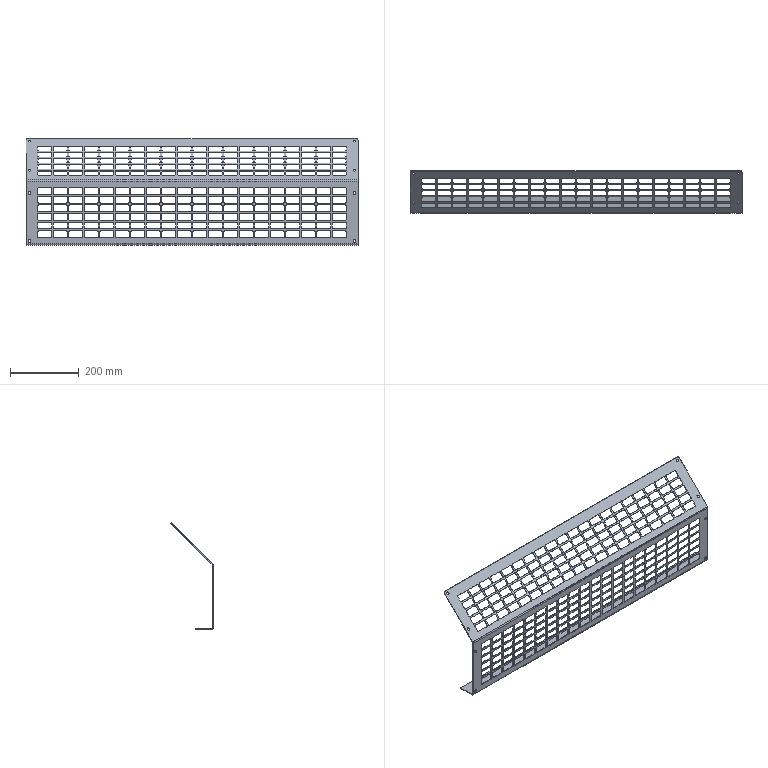Part | STEP file | SYL_0392D6J1SYL0380DJ100-170263 | 1 solid | 1800 faces | box 964 x 122.208 x 308.622 mm | volume 430080 mm3 | cylinder 902 | plane 898 | commonest cylinder face diameters 5 x880 8 x17 10 x2 4 x1 7 x1 11 x1